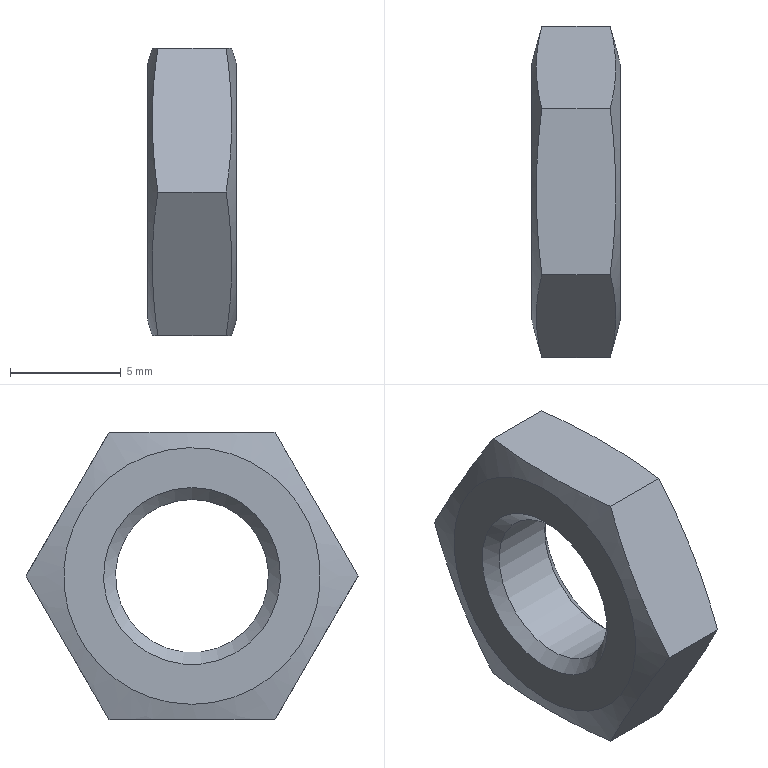Part | NX | features BREP 1 | 1 solid | 13 faces | box 4 x 15.011 x 13 mm | volume 414.331 mm3 | plane 8 | cone 4 | cylinder 1 | commonest cylinder face diameters 6.917 x1
STEP:
#1=CARTESIAN_POINT('',(0.,0.,-5.8));
#2=VERTEX_POINT('',#1);
#3=CARTESIAN_POINT('',(0.,0.,0.));
#4=DIRECTION('',(1.,0.,0.));
#5=DIRECTION('',(0.,0.,-1.));
#6=AXIS2_PLACEMENT_3D('',#3,#4,#5);
#7=CIRCLE('',#6,5.8);
#8=EDGE_CURVE('',#2,#2,#7,.T.);
#9=ORIENTED_EDGE('',*,*,#8,.F.);
#10=EDGE_LOOP('',(#9));
#11=FACE_BOUND('',#10,.T.);
#12=CARTESIAN_POINT('',(0.,0.,4.));
#13=VERTEX_POINT('',#12);
#14=CARTESIAN_POINT('',(0.,0.,0.));
#15=DIRECTION('',(-1.,0.,0.));
#16=DIRECTION('',(0.,0.,1.));
#17=AXIS2_PLACEMENT_3D('',#14,#15,#16);
#18=CIRCLE('',#17,4.);
#19=EDGE_CURVE('',#13,#13,#18,.T.);
#20=ORIENTED_EDGE('',*,*,#19,.F.);
#21=EDGE_LOOP('',(#20));
#22=FACE_BOUND('',#21,.T.);
#23=CARTESIAN_POINT('',(0.,0.,0.));
#24=DIRECTION('',(1.,0.,0.));
#25=DIRECTION('',(0.,0.,1.));
#26=AXIS2_PLACEMENT_3D('',#23,#24,#25);
#27=PLANE('',#26);
#28=ADVANCED_FACE('',(#11,#22),#27,.F.);
#29=CARTESIAN_POINT('',(0.457,-7.506,-0.000000038));
#30=VERTEX_POINT('',#29);
#31=CARTESIAN_POINT('',(0.457,-3.753,6.5));
#32=VERTEX_POINT('',#31);
#33=CARTESIAN_POINT('',(0.457,-7.506,-0.000000024));
#34=CARTESIAN_POINT('',(0.1218,-6.255,2.167));
#35=CARTESIAN_POINT('',(0.1218,-5.004,4.333));
#36=CARTESIAN_POINT('',(0.457,-3.753,6.5));
#37=B_SPLINE_CURVE_WITH_KNOTS('',3,(#33,#34,#35,#36),.UNSPECIFIED.,.F.,.F.,(4,4),(0.,0.007506),.UNSPECIFIED.);
#38=EDGE_CURVE('',#30,#32,#37,.T.);
#39=ORIENTED_EDGE('',*,*,#38,.T.);
#40=CARTESIAN_POINT('',(0.457,3.753,6.5));
#41=VERTEX_POINT('',#40);
#42=CARTESIAN_POINT('',(0.457,-3.753,6.5));
#43=CARTESIAN_POINT('',(0.1218,-1.251,6.5));
#44=CARTESIAN_POINT('',(0.1218,1.251,6.5));
#45=CARTESIAN_POINT('',(0.457,3.753,6.5));
#46=B_SPLINE_CURVE_WITH_KNOTS('',3,(#42,#43,#44,#45),.UNSPECIFIED.,.F.,.F.,(4,4),(0.,0.007506),.UNSPECIFIED.);
#47=EDGE_CURVE('',#32,#41,#46,.T.);
#48=ORIENTED_EDGE('',*,*,#47,.T.);
#49=CARTESIAN_POINT('',(0.457,7.506,0.000000038));
#50=VERTEX_POINT('',#49);
#51=CARTESIAN_POINT('',(0.457,3.753,6.5));
#52=CARTESIAN_POINT('',(0.1218,5.004,4.333));
#53=CARTESIAN_POINT('',(0.1218,6.255,2.167));
#54=CARTESIAN_POINT('',(0.457,7.506,0.000000051));
#55=B_SPLINE_CURVE_WITH_KNOTS('',3,(#51,#52,#53,#54),.UNSPECIFIED.,.F.,.F.,(4,4),(0.,0.007506),.UNSPECIFIED.);
#56=EDGE_CURVE('',#41,#50,#55,.T.);
#57=ORIENTED_EDGE('',*,*,#56,.T.);
#58=CARTESIAN_POINT('',(0.457,3.753,-6.5));
#59=VERTEX_POINT('',#58);
#60=CARTESIAN_POINT('',(0.457,7.506,0.000000024));
#61=CARTESIAN_POINT('',(0.1218,6.255,-2.167));
#62=CARTESIAN_POINT('',(0.1218,5.004,-4.333));
#63=CARTESIAN_POINT('',(0.457,3.753,-6.5));
#64=B_SPLINE_CURVE_WITH_KNOTS('',3,(#60,#61,#62,#63),.UNSPECIFIED.,.F.,.F.,(4,4),(0.,0.007506),.UNSPECIFIED.);
#65=EDGE_CURVE('',#50,#59,#64,.T.);
#66=ORIENTED_EDGE('',*,*,#65,.T.);
#67=CARTESIAN_POINT('',(0.457,-3.753,-6.5));
#68=VERTEX_POINT('',#67);
#69=CARTESIAN_POINT('',(0.457,3.753,-6.5));
#70=CARTESIAN_POINT('',(0.1218,1.251,-6.5));
#71=CARTESIAN_POINT('',(0.1218,-1.251,-6.5));
#72=CARTESIAN_POINT('',(0.457,-3.753,-6.5));
#73=B_SPLINE_CURVE_WITH_KNOTS('',3,(#69,#70,#71,#72),.UNSPECIFIED.,.F.,.F.,(4,4),(0.,0.007506),.UNSPECIFIED.);
#74=EDGE_CURVE('',#59,#68,#73,.T.);
#75=ORIENTED_EDGE('',*,*,#74,.T.);
#76=CARTESIAN_POINT('',(0.457,-3.753,-6.5));
#77=CARTESIAN_POINT('',(0.1218,-5.004,-4.333));
#78=CARTESIAN_POINT('',(0.1218,-6.255,-2.167));
#79=CARTESIAN_POINT('',(0.457,-7.506,-0.000000051));
#80=B_SPLINE_CURVE_WITH_KNOTS('',3,(#76,#77,#78,#79),.UNSPECIFIED.,.F.,.F.,(4,4),(0.,0.007506),.UNSPECIFIED.);
#81=EDGE_CURVE('',#68,#30,#80,.T.);
#82=ORIENTED_EDGE('',*,*,#81,.T.);
#83=EDGE_LOOP('',(#39,#48,#57,#66,#75,#82));
#84=FACE_BOUND('',#83,.T.);
#85=ORIENTED_EDGE('',*,*,#8,.T.);
#86=EDGE_LOOP('',(#85));
#87=FACE_BOUND('',#86,.T.);
#88=CARTESIAN_POINT('',(0.4597,0.,0.));
#89=DIRECTION('',(1.,0.,0.));
#90=DIRECTION('',(0.,0.,1.));
#91=AXIS2_PLACEMENT_3D('',#88,#89,#90);
#92=CONICAL_SURFACE('',#91,7.516,1.309);
#93=ADVANCED_FACE('',(#84,#87),#92,.T.);
#94=ORIENTED_EDGE('',*,*,#19,.T.);
#95=EDGE_LOOP('',(#94));
#96=FACE_BOUND('',#95,.T.);
#97=CARTESIAN_POINT('',(0.5415,0.,3.459));
#98=VERTEX_POINT('',#97);
#99=CARTESIAN_POINT('',(0.5415,0.,0.));
#100=DIRECTION('',(-1.,0.,0.));
#101=DIRECTION('',(0.,0.,1.));
#102=AXIS2_PLACEMENT_3D('',#99,#100,#101);
#103=CIRCLE('',#102,3.459);
#104=EDGE_CURVE('',#98,#98,#103,.T.);
#105=ORIENTED_EDGE('',*,*,#104,.F.);
#106=EDGE_LOOP('',(#105));
#107=FACE_BOUND('',#106,.T.);
#108=CARTESIAN_POINT('',(0.,0.,0.));
#109=DIRECTION('',(-1.,0.,0.));
#110=DIRECTION('',(0.,0.,-1.));
#111=AXIS2_PLACEMENT_3D('',#108,#109,#110);
#112=CONICAL_SURFACE('',#111,4.,0.7854);
#113=ADVANCED_FACE('',(#96,#107),#112,.F.);
#114=CARTESIAN_POINT('',(3.543,-3.753,-6.5));
#115=VERTEX_POINT('',#114);
#116=CARTESIAN_POINT('',(3.543,3.753,-6.5));
#117=VERTEX_POINT('',#116);
#118=CARTESIAN_POINT('',(3.543,-3.753,-6.5));
#119=CARTESIAN_POINT('',(3.878,-1.251,-6.5));
#120=CARTESIAN_POINT('',(3.878,1.251,-6.5));
#121=CARTESIAN_POINT('',(3.543,3.753,-6.5));
#122=B_SPLINE_CURVE_WITH_KNOTS('',3,(#118,#119,#120,#121),.UNSPECIFIED.,.F.,.F.,(4,4),(0.,0.007506),.UNSPECIFIED.);
#123=EDGE_CURVE('',#115,#117,#122,.T.);
#124=ORIENTED_EDGE('',*,*,#123,.F.);
#125=CARTESIAN_POINT('',(4.,-3.753,-6.5));
#126=DIRECTION('',(1.,0.,0.));
#127=VECTOR('',#126,1000.);
#128=LINE('',#125,#127);
#129=EDGE_CURVE('',#68,#115,#128,.T.);
#130=ORIENTED_EDGE('',*,*,#129,.F.);
#131=ORIENTED_EDGE('',*,*,#74,.F.);
#132=CARTESIAN_POINT('',(4.,3.753,-6.5));
#133=DIRECTION('',(-1.,0.,0.));
#134=VECTOR('',#133,1000.);
#135=LINE('',#132,#134);
#136=EDGE_CURVE('',#117,#59,#135,.T.);
#137=ORIENTED_EDGE('',*,*,#136,.F.);
#138=EDGE_LOOP('',(#124,#130,#131,#137));
#139=FACE_BOUND('',#138,.T.);
#140=CARTESIAN_POINT('',(4.,-3.753,-6.5));
#141=DIRECTION('',(0.,0.,1.));
#142=DIRECTION('',(-1.,0.,0.));
#143=AXIS2_PLACEMENT_3D('',#140,#141,#142);
#144=PLANE('',#143);
#145=ADVANCED_FACE('',(#139),#144,.F.);
#146=CARTESIAN_POINT('',(3.543,7.506,0.));
#147=VERTEX_POINT('',#146);
#148=CARTESIAN_POINT('',(3.543,3.753,-6.5));
#149=CARTESIAN_POINT('',(3.878,5.004,-4.333));
#150=CARTESIAN_POINT('',(3.878,6.255,-2.167));
#151=CARTESIAN_POINT('',(3.543,7.506,0.));
#152=B_SPLINE_CURVE_WITH_KNOTS('',3,(#148,#149,#150,#151),.UNSPECIFIED.,.F.,.F.,(4,4),(0.,0.007506),.UNSPECIFIED.);
#153=EDGE_CURVE('',#117,#147,#152,.T.);
#154=ORIENTED_EDGE('',*,*,#153,.F.);
#155=ORIENTED_EDGE('',*,*,#136,.T.);
#156=ORIENTED_EDGE('',*,*,#65,.F.);
#157=CARTESIAN_POINT('',(4.,7.506,0.));
#158=DIRECTION('',(-1.,0.,0.));
#159=VECTOR('',#158,1000.);
#160=LINE('',#157,#159);
#161=EDGE_CURVE('',#147,#50,#160,.T.);
#162=ORIENTED_EDGE('',*,*,#161,.F.);
#163=EDGE_LOOP('',(#154,#155,#156,#162));
#164=FACE_BOUND('',#163,.T.);
#165=CARTESIAN_POINT('',(4.,3.753,-6.5));
#166=DIRECTION('',(0.,-0.866,0.5));
#167=DIRECTION('',(0.,0.5,0.866));
#168=AXIS2_PLACEMENT_3D('',#165,#166,#167);
#169=PLANE('',#168);
#170=ADVANCED_FACE('',(#164),#169,.F.);
#171=CARTESIAN_POINT('',(3.543,3.753,6.5));
#172=VERTEX_POINT('',#171);
#173=CARTESIAN_POINT('',(3.543,7.506,0.));
#174=CARTESIAN_POINT('',(3.878,6.255,2.167));
#175=CARTESIAN_POINT('',(3.878,5.004,4.333));
#176=CARTESIAN_POINT('',(3.543,3.753,6.5));
#177=B_SPLINE_CURVE_WITH_KNOTS('',3,(#173,#174,#175,#176),.UNSPECIFIED.,.F.,.F.,(4,4),(0.,0.007506),.UNSPECIFIED.);
#178=EDGE_CURVE('',#147,#172,#177,.T.);
#179=ORIENTED_EDGE('',*,*,#178,.F.);
#180=ORIENTED_EDGE('',*,*,#161,.T.);
#181=ORIENTED_EDGE('',*,*,#56,.F.);
#182=CARTESIAN_POINT('',(4.,3.753,6.5));
#183=DIRECTION('',(-1.,0.,0.));
#184=VECTOR('',#183,1000.);
#185=LINE('',#182,#184);
#186=EDGE_CURVE('',#172,#41,#185,.T.);
#187=ORIENTED_EDGE('',*,*,#186,.F.);
#188=EDGE_LOOP('',(#179,#180,#181,#187));
#189=FACE_BOUND('',#188,.T.);
#190=CARTESIAN_POINT('',(4.,7.506,0.));
#191=DIRECTION('',(0.,-0.866,-0.5));
#192=DIRECTION('',(0.,-0.5,0.866));
#193=AXIS2_PLACEMENT_3D('',#190,#191,#192);
#194=PLANE('',#193);
#195=ADVANCED_FACE('',(#189),#194,.F.);
#196=CARTESIAN_POINT('',(3.543,-3.753,6.5));
#197=VERTEX_POINT('',#196);
#198=CARTESIAN_POINT('',(3.543,3.753,6.5));
#199=CARTESIAN_POINT('',(3.878,1.251,6.5));
#200=CARTESIAN_POINT('',(3.878,-1.251,6.5));
#201=CARTESIAN_POINT('',(3.543,-3.753,6.5));
#202=B_SPLINE_CURVE_WITH_KNOTS('',3,(#198,#199,#200,#201),.UNSPECIFIED.,.F.,.F.,(4,4),(0.,0.007506),.UNSPECIFIED.);
#203=EDGE_CURVE('',#172,#197,#202,.T.);
#204=ORIENTED_EDGE('',*,*,#203,.F.);
#205=ORIENTED_EDGE('',*,*,#186,.T.);
#206=ORIENTED_EDGE('',*,*,#47,.F.);
#207=CARTESIAN_POINT('',(4.,-3.753,6.5));
#208=DIRECTION('',(-1.,0.,0.));
#209=VECTOR('',#208,1000.);
#210=LINE('',#207,#209);
#211=EDGE_CURVE('',#197,#32,#210,.T.);
#212=ORIENTED_EDGE('',*,*,#211,.F.);
#213=EDGE_LOOP('',(#204,#205,#206,#212));
#214=FACE_BOUND('',#213,.T.);
#215=CARTESIAN_POINT('',(4.,3.753,6.5));
#216=DIRECTION('',(0.,0.,-1.));
#217=DIRECTION('',(1.,0.,0.));
#218=AXIS2_PLACEMENT_3D('',#215,#216,#217);
#219=PLANE('',#218);
#220=ADVANCED_FACE('',(#214),#219,.F.);
#221=CARTESIAN_POINT('',(3.543,-7.506,0.));
#222=VERTEX_POINT('',#221);
#223=CARTESIAN_POINT('',(3.543,-3.753,6.5));
#224=CARTESIAN_POINT('',(3.878,-5.004,4.333));
#225=CARTESIAN_POINT('',(3.878,-6.255,2.167));
#226=CARTESIAN_POINT('',(3.543,-7.506,0.));
#227=B_SPLINE_CURVE_WITH_KNOTS('',3,(#223,#224,#225,#226),.UNSPECIFIED.,.F.,.F.,(4,4),(0.,0.007506),.UNSPECIFIED.);
#228=EDGE_CURVE('',#197,#222,#227,.T.);
#229=ORIENTED_EDGE('',*,*,#228,.F.);
#230=ORIENTED_EDGE('',*,*,#211,.T.);
#231=ORIENTED_EDGE('',*,*,#38,.F.);
#232=CARTESIAN_POINT('',(4.,-7.506,0.));
#233=DIRECTION('',(-1.,0.,0.));
#234=VECTOR('',#233,1000.);
#235=LINE('',#232,#234);
#236=EDGE_CURVE('',#222,#30,#235,.T.);
#237=ORIENTED_EDGE('',*,*,#236,.F.);
#238=EDGE_LOOP('',(#229,#230,#231,#237));
#239=FACE_BOUND('',#238,.T.);
#240=CARTESIAN_POINT('',(4.,-3.753,6.5));
#241=DIRECTION('',(0.,0.866,-0.5));
#242=DIRECTION('',(0.,-0.5,-0.866));
#243=AXIS2_PLACEMENT_3D('',#240,#241,#242);
#244=PLANE('',#243);
#245=ADVANCED_FACE('',(#239),#244,.F.);
#246=CARTESIAN_POINT('',(3.543,-7.506,0.));
#247=CARTESIAN_POINT('',(3.878,-6.255,-2.167));
#248=CARTESIAN_POINT('',(3.878,-5.004,-4.333));
#249=CARTESIAN_POINT('',(3.543,-3.753,-6.5));
#250=B_SPLINE_CURVE_WITH_KNOTS('',3,(#246,#247,#248,#249),.UNSPECIFIED.,.F.,.F.,(4,4),(0.,0.007506),.UNSPECIFIED.);
#251=EDGE_CURVE('',#222,#115,#250,.T.);
#252=ORIENTED_EDGE('',*,*,#251,.F.);
#253=ORIENTED_EDGE('',*,*,#236,.T.);
#254=ORIENTED_EDGE('',*,*,#81,.F.);
#255=ORIENTED_EDGE('',*,*,#129,.T.);
#256=EDGE_LOOP('',(#252,#253,#254,#255));
#257=FACE_BOUND('',#256,.T.);
#258=CARTESIAN_POINT('',(4.,-7.506,0.));
#259=DIRECTION('',(0.,0.866,0.5));
#260=DIRECTION('',(0.,0.5,-0.866));
#261=AXIS2_PLACEMENT_3D('',#258,#259,#260);
#262=PLANE('',#261);
#263=ADVANCED_FACE('',(#257),#262,.F.);
#264=CARTESIAN_POINT('',(3.458,0.,3.458));
#265=VERTEX_POINT('',#264);
#266=CARTESIAN_POINT('',(3.458,0.,0.));
#267=DIRECTION('',(-1.,0.,0.));
#268=DIRECTION('',(0.,0.,1.));
#269=AXIS2_PLACEMENT_3D('',#266,#267,#268);
#270=CIRCLE('',#269,3.458);
#271=EDGE_CURVE('',#265,#265,#270,.T.);
#272=ORIENTED_EDGE('',*,*,#271,.F.);
#273=EDGE_LOOP('',(#272));
#274=FACE_BOUND('',#273,.T.);
#275=ORIENTED_EDGE('',*,*,#104,.T.);
#276=EDGE_LOOP('',(#275));
#277=FACE_BOUND('',#276,.T.);
#278=CARTESIAN_POINT('',(4.,0.,0.));
#279=DIRECTION('',(-1.,0.,0.));
#280=DIRECTION('',(0.,0.,-1.));
#281=AXIS2_PLACEMENT_3D('',#278,#279,#280);
#282=CYLINDRICAL_SURFACE('',#281,3.458);
#283=ADVANCED_FACE('',(#274,#277),#282,.F.);
#284=ORIENTED_EDGE('',*,*,#251,.T.);
#285=ORIENTED_EDGE('',*,*,#123,.T.);
#286=ORIENTED_EDGE('',*,*,#153,.T.);
#287=ORIENTED_EDGE('',*,*,#178,.T.);
#288=ORIENTED_EDGE('',*,*,#203,.T.);
#289=ORIENTED_EDGE('',*,*,#228,.T.);
#290=EDGE_LOOP('',(#284,#285,#286,#287,#288,#289));
#291=FACE_BOUND('',#290,.T.);
#292=CARTESIAN_POINT('',(4.,0.,5.8));
#293=VERTEX_POINT('',#292);
#294=CARTESIAN_POINT('',(4.,0.,0.));
#295=DIRECTION('',(-1.,0.,0.));
#296=DIRECTION('',(0.,0.,1.));
#297=AXIS2_PLACEMENT_3D('',#294,#295,#296);
#298=CIRCLE('',#297,5.8);
#299=EDGE_CURVE('',#293,#293,#298,.T.);
#300=ORIENTED_EDGE('',*,*,#299,.T.);
#301=EDGE_LOOP('',(#300));
#302=FACE_BOUND('',#301,.T.);
#303=CARTESIAN_POINT('',(3.54,0.,0.));
#304=DIRECTION('',(-1.,0.,0.));
#305=DIRECTION('',(0.,0.,-1.));
#306=AXIS2_PLACEMENT_3D('',#303,#304,#305);
#307=CONICAL_SURFACE('',#306,7.516,1.309);
#308=ADVANCED_FACE('',(#291,#302),#307,.T.);
#309=CARTESIAN_POINT('',(4.,0.,-4.));
#310=VERTEX_POINT('',#309);
#311=CARTESIAN_POINT('',(4.,0.,0.));
#312=DIRECTION('',(-1.,0.,0.));
#313=DIRECTION('',(0.,0.,-1.));
#314=AXIS2_PLACEMENT_3D('',#311,#312,#313);
#315=CIRCLE('',#314,4.);
#316=EDGE_CURVE('',#310,#310,#315,.T.);
#317=ORIENTED_EDGE('',*,*,#316,.F.);
#318=EDGE_LOOP('',(#317));
#319=FACE_BOUND('',#318,.T.);
#320=ORIENTED_EDGE('',*,*,#271,.T.);
#321=EDGE_LOOP('',(#320));
#322=FACE_BOUND('',#321,.T.);
#323=CARTESIAN_POINT('',(4.,0.,0.));
#324=DIRECTION('',(1.,0.,0.));
#325=DIRECTION('',(0.,0.,1.));
#326=AXIS2_PLACEMENT_3D('',#323,#324,#325);
#327=CONICAL_SURFACE('',#326,4.,0.7854);
#328=ADVANCED_FACE('',(#319,#322),#327,.F.);
#329=ORIENTED_EDGE('',*,*,#299,.F.);
#330=EDGE_LOOP('',(#329));
#331=FACE_BOUND('',#330,.T.);
#332=ORIENTED_EDGE('',*,*,#316,.T.);
#333=EDGE_LOOP('',(#332));
#334=FACE_BOUND('',#333,.T.);
#335=CARTESIAN_POINT('',(4.,5.8,0.));
#336=DIRECTION('',(-1.,0.,0.));
#337=DIRECTION('',(0.,0.,-1.));
#338=AXIS2_PLACEMENT_3D('',#335,#336,#337);
#339=PLANE('',#338);
#340=ADVANCED_FACE('',(#331,#334),#339,.F.);
#341=CLOSED_SHELL('',(#28,#93,#113,#145,#170,#195,#220,#245,#263,#283,#308,#328,#340));
#342=MANIFOLD_SOLID_BREP('',#341);
#343=(LENGTH_UNIT()NAMED_UNIT(*)SI_UNIT(.MILLI.,.METRE.));
#344=UNCERTAINTY_MEASURE_WITH_UNIT(LENGTH_MEASURE(0.0508),#343,'','');
#345=(NAMED_UNIT(*)PLANE_ANGLE_UNIT()SI_UNIT($,.RADIAN.));
#346=(NAMED_UNIT(*)SI_UNIT($,.STERADIAN.)SOLID_ANGLE_UNIT());
#347=(GEOMETRIC_REPRESENTATION_CONTEXT(3)GLOBAL_UNCERTAINTY_ASSIGNED_CONTEXT((#344))GLOBAL_UNIT_ASSIGNED_CONTEXT((#343,#345,#346))REPRESENTATION_CONTEXT('',''));
#348=ADVANCED_BREP_SHAPE_REPRESENTATION('',(#342),#347);